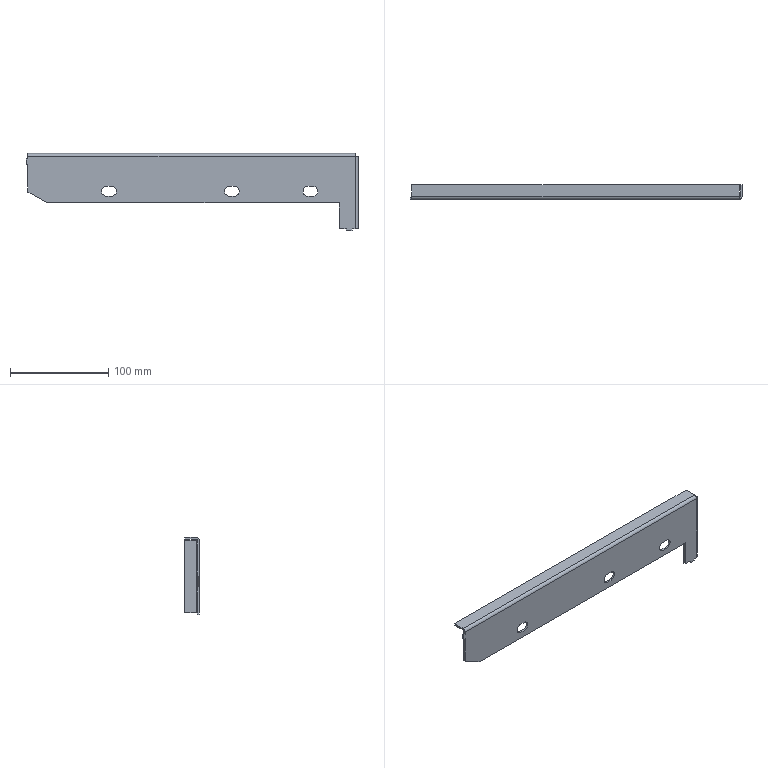Part | SolidWorks | features ICE 3, Cut 2, EdgeFlange 2, FlatPattern 1, SMBaseFlange 1, SheetMetal 1 | 1 solid | 45 faces | box 338 x 15 x 78.5 mm | volume 43707 mm3 | plane 35 | cylinder 10 | commonest cylinder face diameters 10 x6 2 x2 6 x2
STEP:
#1=CARTESIAN_POINT('',(-16.,0.,0.));
#2=VERTEX_POINT('',#1);
#3=CARTESIAN_POINT('',(-9.,0.,0.));
#4=VERTEX_POINT('',#3);
#5=CARTESIAN_POINT('',(-333.,0.,0.));
#6=DIRECTION('',(1.,0.,0.));
#7=VECTOR('',#6,1000.);
#8=LINE('',#5,#7);
#9=EDGE_CURVE('',#2,#4,#8,.T.);
#10=ORIENTED_EDGE('',*,*,#9,.T.);
#11=CARTESIAN_POINT('',(-9.,-2.,0.));
#12=VERTEX_POINT('',#11);
#13=CARTESIAN_POINT('',(-9.,0.,0.));
#14=DIRECTION('',(0.,1.,0.));
#15=VECTOR('',#14,1000.);
#16=LINE('',#13,#15);
#17=EDGE_CURVE('',#12,#4,#16,.T.);
#18=ORIENTED_EDGE('',*,*,#17,.F.);
#19=CARTESIAN_POINT('',(-16.,-2.,0.));
#20=VERTEX_POINT('',#19);
#21=CARTESIAN_POINT('',(-333.,-2.,0.));
#22=DIRECTION('',(1.,0.,0.));
#23=VECTOR('',#22,1000.);
#24=LINE('',#21,#23);
#25=EDGE_CURVE('',#20,#12,#24,.T.);
#26=ORIENTED_EDGE('',*,*,#25,.F.);
#27=CARTESIAN_POINT('',(-16.,0.,0.));
#28=DIRECTION('',(0.,-1.,0.));
#29=VECTOR('',#28,1000.);
#30=LINE('',#27,#29);
#31=EDGE_CURVE('',#2,#20,#30,.T.);
#32=ORIENTED_EDGE('',*,*,#31,.F.);
#33=EDGE_LOOP('',(#10,#18,#26,#32));
#34=FACE_OUTER_BOUND('',#33,.T.);
#35=CARTESIAN_POINT('',(0.,0.,0.));
#36=DIRECTION('',(0.,0.,-1.));
#37=DIRECTION('',(-1.,0.,0.));
#38=AXIS2_PLACEMENT_3D('',#35,#36,#37);
#39=PLANE('',#38);
#40=ADVANCED_FACE('',(#34),#39,.T.);
#41=CARTESIAN_POINT('',(-3.,-2.,0.));
#42=VERTEX_POINT('',#41);
#43=CARTESIAN_POINT('',(0.,-2.,0.));
#44=VERTEX_POINT('',#43);
#45=CARTESIAN_POINT('',(-333.,-2.,0.));
#46=DIRECTION('',(1.,0.,0.));
#47=VECTOR('',#46,1000.);
#48=LINE('',#45,#47);
#49=EDGE_CURVE('',#42,#44,#48,.T.);
#50=ORIENTED_EDGE('',*,*,#49,.F.);
#51=CARTESIAN_POINT('',(-3.,0.,0.));
#52=VERTEX_POINT('',#51);
#53=CARTESIAN_POINT('',(-3.,0.,0.));
#54=DIRECTION('',(0.,-1.,0.));
#55=VECTOR('',#54,1000.);
#56=LINE('',#53,#55);
#57=EDGE_CURVE('',#52,#42,#56,.T.);
#58=ORIENTED_EDGE('',*,*,#57,.F.);
#59=CARTESIAN_POINT('',(0.,0.,0.));
#60=VERTEX_POINT('',#59);
#61=CARTESIAN_POINT('',(-333.,0.,0.));
#62=DIRECTION('',(1.,0.,0.));
#63=VECTOR('',#62,1000.);
#64=LINE('',#61,#63);
#65=EDGE_CURVE('',#52,#60,#64,.T.);
#66=ORIENTED_EDGE('',*,*,#65,.T.);
#67=CARTESIAN_POINT('',(0.,0.,0.));
#68=DIRECTION('',(0.,-1.,0.));
#69=VECTOR('',#68,1000.);
#70=LINE('',#67,#69);
#71=EDGE_CURVE('',#60,#44,#70,.T.);
#72=ORIENTED_EDGE('',*,*,#71,.T.);
#73=EDGE_LOOP('',(#50,#58,#66,#72));
#74=FACE_OUTER_BOUND('',#73,.T.);
#75=CARTESIAN_POINT('',(0.,0.,0.));
#76=DIRECTION('',(0.,0.,-1.));
#77=DIRECTION('',(-1.,0.,0.));
#78=AXIS2_PLACEMENT_3D('',#75,#76,#77);
#79=PLANE('',#78);
#80=ADVANCED_FACE('',(#74),#79,.T.);
#81=CARTESIAN_POINT('',(-333.,0.,73.5));
#82=VERTEX_POINT('',#81);
#83=CARTESIAN_POINT('',(-333.,0.,71.));
#84=VERTEX_POINT('',#83);
#85=CARTESIAN_POINT('',(-333.,0.,73.5));
#86=DIRECTION('',(0.,0.,-1.));
#87=VECTOR('',#86,1000.);
#88=LINE('',#85,#87);
#89=EDGE_CURVE('',#82,#84,#88,.T.);
#90=ORIENTED_EDGE('',*,*,#89,.T.);
#91=CARTESIAN_POINT('',(-333.,-2.,71.));
#92=VERTEX_POINT('',#91);
#93=CARTESIAN_POINT('',(-333.,-2.,71.));
#94=DIRECTION('',(0.,1.,0.));
#95=VECTOR('',#94,1000.);
#96=LINE('',#93,#95);
#97=EDGE_CURVE('',#92,#84,#96,.T.);
#98=ORIENTED_EDGE('',*,*,#97,.F.);
#99=CARTESIAN_POINT('',(-333.,-2.,73.5));
#100=VERTEX_POINT('',#99);
#101=CARTESIAN_POINT('',(-333.,-2.,73.5));
#102=DIRECTION('',(0.,0.,-1.));
#103=VECTOR('',#102,1000.);
#104=LINE('',#101,#103);
#105=EDGE_CURVE('',#100,#92,#104,.T.);
#106=ORIENTED_EDGE('',*,*,#105,.F.);
#107=CARTESIAN_POINT('',(-333.,-2.,73.5));
#108=DIRECTION('',(0.,1.,0.));
#109=VECTOR('',#108,1000.);
#110=LINE('',#107,#109);
#111=EDGE_CURVE('',#100,#82,#110,.T.);
#112=ORIENTED_EDGE('',*,*,#111,.T.);
#113=EDGE_LOOP('',(#90,#98,#106,#112));
#114=FACE_OUTER_BOUND('',#113,.T.);
#115=CARTESIAN_POINT('',(-333.,-2.,73.5));
#116=DIRECTION('',(-1.,0.,0.));
#117=DIRECTION('',(0.,0.,1.));
#118=AXIS2_PLACEMENT_3D('',#115,#116,#117);
#119=PLANE('',#118);
#120=ADVANCED_FACE('',(#114),#119,.T.);
#121=CARTESIAN_POINT('',(-333.,-2.,65.));
#122=VERTEX_POINT('',#121);
#123=CARTESIAN_POINT('',(-333.,-2.,37.2));
#124=VERTEX_POINT('',#123);
#125=CARTESIAN_POINT('',(-333.,-2.,73.5));
#126=DIRECTION('',(0.,0.,-1.));
#127=VECTOR('',#126,1000.);
#128=LINE('',#125,#127);
#129=EDGE_CURVE('',#122,#124,#128,.T.);
#130=ORIENTED_EDGE('',*,*,#129,.F.);
#131=CARTESIAN_POINT('',(-333.,0.,65.));
#132=VERTEX_POINT('',#131);
#133=CARTESIAN_POINT('',(-333.,-2.,65.));
#134=DIRECTION('',(0.,-1.,0.));
#135=VECTOR('',#134,1000.);
#136=LINE('',#133,#135);
#137=EDGE_CURVE('',#132,#122,#136,.T.);
#138=ORIENTED_EDGE('',*,*,#137,.F.);
#139=CARTESIAN_POINT('',(-333.,0.,37.2));
#140=VERTEX_POINT('',#139);
#141=CARTESIAN_POINT('',(-333.,0.,73.5));
#142=DIRECTION('',(0.,0.,-1.));
#143=VECTOR('',#142,1000.);
#144=LINE('',#141,#143);
#145=EDGE_CURVE('',#132,#140,#144,.T.);
#146=ORIENTED_EDGE('',*,*,#145,.T.);
#147=CARTESIAN_POINT('',(-333.,8.,37.2));
#148=DIRECTION('',(0.,-1.,0.));
#149=VECTOR('',#148,1000.);
#150=LINE('',#147,#149);
#151=EDGE_CURVE('',#140,#124,#150,.T.);
#152=ORIENTED_EDGE('',*,*,#151,.T.);
#153=EDGE_LOOP('',(#130,#138,#146,#152));
#154=FACE_OUTER_BOUND('',#153,.T.);
#155=CARTESIAN_POINT('',(-333.,-2.,73.5));
#156=DIRECTION('',(-1.,0.,0.));
#157=DIRECTION('',(0.,0.,1.));
#158=AXIS2_PLACEMENT_3D('',#155,#156,#157);
#159=PLANE('',#158);
#160=ADVANCED_FACE('',(#154),#159,.T.);
#161=CARTESIAN_POINT('',(-253.,-2.,33.));
#162=VERTEX_POINT('',#161);
#163=CARTESIAN_POINT('',(-248.,-2.,33.));
#164=VERTEX_POINT('',#163);
#165=CARTESIAN_POINT('',(-253.,-2.,33.));
#166=DIRECTION('',(1.,0.,0.));
#167=VECTOR('',#166,1000.);
#168=LINE('',#165,#167);
#169=EDGE_CURVE('',#162,#164,#168,.T.);
#170=ORIENTED_EDGE('',*,*,#169,.F.);
#171=CARTESIAN_POINT('',(-253.,-2.,43.));
#172=VERTEX_POINT('',#171);
#173=CARTESIAN_POINT('',(-253.,-2.,38.));
#174=DIRECTION('',(0.,-1.,0.));
#175=DIRECTION('',(0.,0.,-1.));
#176=AXIS2_PLACEMENT_3D('',#173,#174,#175);
#177=CIRCLE('',#176,5.);
#178=EDGE_CURVE('',#172,#162,#177,.T.);
#179=ORIENTED_EDGE('',*,*,#178,.F.);
#180=CARTESIAN_POINT('',(-248.,-2.,43.));
#181=VERTEX_POINT('',#180);
#182=CARTESIAN_POINT('',(-253.,-2.,43.));
#183=DIRECTION('',(-1.,0.,0.));
#184=VECTOR('',#183,1000.);
#185=LINE('',#182,#184);
#186=EDGE_CURVE('',#181,#172,#185,.T.);
#187=ORIENTED_EDGE('',*,*,#186,.F.);
#188=CARTESIAN_POINT('',(-248.,-2.,38.));
#189=DIRECTION('',(0.,-1.,0.));
#190=DIRECTION('',(0.,0.,-1.));
#191=AXIS2_PLACEMENT_3D('',#188,#189,#190);
#192=CIRCLE('',#191,5.);
#193=EDGE_CURVE('',#164,#181,#192,.T.);
#194=ORIENTED_EDGE('',*,*,#193,.F.);
#195=EDGE_LOOP('',(#170,#179,#187,#194));
#196=FACE_BOUND('',#195,.T.);
#197=CARTESIAN_POINT('',(-128.,-2.,33.));
#198=VERTEX_POINT('',#197);
#199=CARTESIAN_POINT('',(-123.,-2.,33.));
#200=VERTEX_POINT('',#199);
#201=CARTESIAN_POINT('',(-128.,-2.,33.));
#202=DIRECTION('',(1.,0.,0.));
#203=VECTOR('',#202,1000.);
#204=LINE('',#201,#203);
#205=EDGE_CURVE('',#198,#200,#204,.T.);
#206=ORIENTED_EDGE('',*,*,#205,.F.);
#207=CARTESIAN_POINT('',(-128.,-2.,43.));
#208=VERTEX_POINT('',#207);
#209=CARTESIAN_POINT('',(-128.,-2.,38.));
#210=DIRECTION('',(0.,-1.,0.));
#211=DIRECTION('',(0.,0.,-1.));
#212=AXIS2_PLACEMENT_3D('',#209,#210,#211);
#213=CIRCLE('',#212,5.);
#214=EDGE_CURVE('',#208,#198,#213,.T.);
#215=ORIENTED_EDGE('',*,*,#214,.F.);
#216=CARTESIAN_POINT('',(-123.,-2.,43.));
#217=VERTEX_POINT('',#216);
#218=CARTESIAN_POINT('',(-128.,-2.,43.));
#219=DIRECTION('',(-1.,0.,0.));
#220=VECTOR('',#219,1000.);
#221=LINE('',#218,#220);
#222=EDGE_CURVE('',#217,#208,#221,.T.);
#223=ORIENTED_EDGE('',*,*,#222,.F.);
#224=CARTESIAN_POINT('',(-123.,-2.,38.));
#225=DIRECTION('',(0.,-1.,0.));
#226=DIRECTION('',(0.,0.,-1.));
#227=AXIS2_PLACEMENT_3D('',#224,#225,#226);
#228=CIRCLE('',#227,5.);
#229=EDGE_CURVE('',#200,#217,#228,.T.);
#230=ORIENTED_EDGE('',*,*,#229,.F.);
#231=EDGE_LOOP('',(#206,#215,#223,#230));
#232=FACE_BOUND('',#231,.T.);
#233=CARTESIAN_POINT('',(-48.,-2.,33.));
#234=VERTEX_POINT('',#233);
#235=CARTESIAN_POINT('',(-43.,-2.,33.));
#236=VERTEX_POINT('',#235);
#237=CARTESIAN_POINT('',(-48.,-2.,33.));
#238=DIRECTION('',(1.,0.,0.));
#239=VECTOR('',#238,1000.);
#240=LINE('',#237,#239);
#241=EDGE_CURVE('',#234,#236,#240,.T.);
#242=ORIENTED_EDGE('',*,*,#241,.F.);
#243=CARTESIAN_POINT('',(-48.,-2.,43.));
#244=VERTEX_POINT('',#243);
#245=CARTESIAN_POINT('',(-48.,-2.,38.));
#246=DIRECTION('',(0.,-1.,0.));
#247=DIRECTION('',(0.,0.,-1.));
#248=AXIS2_PLACEMENT_3D('',#245,#246,#247);
#249=CIRCLE('',#248,5.);
#250=EDGE_CURVE('',#244,#234,#249,.T.);
#251=ORIENTED_EDGE('',*,*,#250,.F.);
#252=CARTESIAN_POINT('',(-43.,-2.,43.));
#253=VERTEX_POINT('',#252);
#254=CARTESIAN_POINT('',(-48.,-2.,43.));
#255=DIRECTION('',(-1.,0.,0.));
#256=VECTOR('',#255,1000.);
#257=LINE('',#254,#256);
#258=EDGE_CURVE('',#253,#244,#257,.T.);
#259=ORIENTED_EDGE('',*,*,#258,.F.);
#260=CARTESIAN_POINT('',(-43.,-2.,38.));
#261=DIRECTION('',(0.,-1.,0.));
#262=DIRECTION('',(0.,0.,-1.));
#263=AXIS2_PLACEMENT_3D('',#260,#261,#262);
#264=CIRCLE('',#263,5.);
#265=EDGE_CURVE('',#236,#253,#264,.T.);
#266=ORIENTED_EDGE('',*,*,#265,.F.);
#267=EDGE_LOOP('',(#242,#251,#259,#266));
#268=FACE_BOUND('',#267,.T.);
#269=ORIENTED_EDGE('',*,*,#105,.T.);
#270=CARTESIAN_POINT('',(-335.,-2.,71.));
#271=VERTEX_POINT('',#270);
#272=CARTESIAN_POINT('',(-335.,-2.,71.));
#273=DIRECTION('',(1.,0.,0.));
#274=VECTOR('',#273,1000.);
#275=LINE('',#272,#274);
#276=EDGE_CURVE('',#271,#92,#275,.T.);
#277=ORIENTED_EDGE('',*,*,#276,.F.);
#278=CARTESIAN_POINT('',(-335.,-2.,65.));
#279=VERTEX_POINT('',#278);
#280=CARTESIAN_POINT('',(-335.,-2.,71.));
#281=DIRECTION('',(0.,0.,1.));
#282=VECTOR('',#281,1000.);
#283=LINE('',#280,#282);
#284=EDGE_CURVE('',#279,#271,#283,.T.);
#285=ORIENTED_EDGE('',*,*,#284,.F.);
#286=CARTESIAN_POINT('',(-335.,-2.,65.));
#287=DIRECTION('',(1.,0.,0.));
#288=VECTOR('',#287,1000.);
#289=LINE('',#286,#288);
#290=EDGE_CURVE('',#279,#122,#289,.T.);
#291=ORIENTED_EDGE('',*,*,#290,.T.);
#292=ORIENTED_EDGE('',*,*,#129,.T.);
#293=CARTESIAN_POINT('',(-313.,-2.,26.2));
#294=VERTEX_POINT('',#293);
#295=CARTESIAN_POINT('',(-333.,-2.,37.2));
#296=DIRECTION('',(-0.8762,0.,0.4819));
#297=VECTOR('',#296,1000.);
#298=LINE('',#295,#297);
#299=EDGE_CURVE('',#294,#124,#298,.T.);
#300=ORIENTED_EDGE('',*,*,#299,.F.);
#301=CARTESIAN_POINT('',(-16.,-2.,26.2));
#302=VERTEX_POINT('',#301);
#303=CARTESIAN_POINT('',(-333.,-2.,26.2));
#304=DIRECTION('',(-1.,0.,0.));
#305=VECTOR('',#304,1000.);
#306=LINE('',#303,#305);
#307=EDGE_CURVE('',#302,#294,#306,.T.);
#308=ORIENTED_EDGE('',*,*,#307,.F.);
#309=CARTESIAN_POINT('',(-16.,-2.,0.));
#310=DIRECTION('',(0.,0.,1.));
#311=VECTOR('',#310,1000.);
#312=LINE('',#309,#311);
#313=EDGE_CURVE('',#20,#302,#312,.T.);
#314=ORIENTED_EDGE('',*,*,#313,.F.);
#315=ORIENTED_EDGE('',*,*,#25,.T.);
#316=CARTESIAN_POINT('',(-9.,-2.,-2.));
#317=VERTEX_POINT('',#316);
#318=CARTESIAN_POINT('',(-9.,-2.,-2.));
#319=DIRECTION('',(0.,0.,1.));
#320=VECTOR('',#319,1000.);
#321=LINE('',#318,#320);
#322=EDGE_CURVE('',#317,#12,#321,.T.);
#323=ORIENTED_EDGE('',*,*,#322,.F.);
#324=CARTESIAN_POINT('',(-3.,-2.,-2.));
#325=VERTEX_POINT('',#324);
#326=CARTESIAN_POINT('',(-9.,-2.,-2.));
#327=DIRECTION('',(-1.,0.,0.));
#328=VECTOR('',#327,1000.);
#329=LINE('',#326,#328);
#330=EDGE_CURVE('',#325,#317,#329,.T.);
#331=ORIENTED_EDGE('',*,*,#330,.F.);
#332=CARTESIAN_POINT('',(-3.,-2.,-2.));
#333=DIRECTION('',(0.,0.,1.));
#334=VECTOR('',#333,1000.);
#335=LINE('',#332,#334);
#336=EDGE_CURVE('',#325,#42,#335,.T.);
#337=ORIENTED_EDGE('',*,*,#336,.T.);
#338=ORIENTED_EDGE('',*,*,#49,.T.);
#339=CARTESIAN_POINT('',(0.,-2.,73.5));
#340=VERTEX_POINT('',#339);
#341=CARTESIAN_POINT('',(0.,-2.,73.5));
#342=DIRECTION('',(0.,0.,-1.));
#343=VECTOR('',#342,1000.);
#344=LINE('',#341,#343);
#345=EDGE_CURVE('',#340,#44,#344,.T.);
#346=ORIENTED_EDGE('',*,*,#345,.F.);
#347=CARTESIAN_POINT('',(-333.,-2.,73.5));
#348=DIRECTION('',(1.,0.,0.));
#349=VECTOR('',#348,1000.);
#350=LINE('',#347,#349);
#351=EDGE_CURVE('',#100,#340,#350,.T.);
#352=ORIENTED_EDGE('',*,*,#351,.F.);
#353=EDGE_LOOP('',(#269,#277,#285,#291,#292,#300,#308,#314,#315,#323,#331,#337,#338,#346,#352));
#354=FACE_OUTER_BOUND('',#353,.T.);
#355=CARTESIAN_POINT('',(-333.,-2.,73.5));
#356=DIRECTION('',(0.,1.,0.));
#357=DIRECTION('',(0.,0.,1.));
#358=AXIS2_PLACEMENT_3D('',#355,#356,#357);
#359=PLANE('',#358);
#360=ADVANCED_FACE('',(#196,#232,#268,#354),#359,.F.);
#361=CARTESIAN_POINT('',(-313.,0.,26.2));
#362=VERTEX_POINT('',#361);
#363=CARTESIAN_POINT('',(-348.328,0.,45.631));
#364=DIRECTION('',(0.8762,0.,-0.4819));
#365=VECTOR('',#364,1000.);
#366=LINE('',#363,#365);
#367=EDGE_CURVE('',#140,#362,#366,.T.);
#368=ORIENTED_EDGE('',*,*,#367,.F.);
#369=ORIENTED_EDGE('',*,*,#145,.F.);
#370=CARTESIAN_POINT('',(-335.,0.,65.));
#371=VERTEX_POINT('',#370);
#372=CARTESIAN_POINT('',(-335.,0.,65.));
#373=DIRECTION('',(1.,0.,0.));
#374=VECTOR('',#373,1000.);
#375=LINE('',#372,#374);
#376=EDGE_CURVE('',#371,#132,#375,.T.);
#377=ORIENTED_EDGE('',*,*,#376,.F.);
#378=CARTESIAN_POINT('',(-335.,0.,71.));
#379=VERTEX_POINT('',#378);
#380=CARTESIAN_POINT('',(-335.,0.,71.));
#381=DIRECTION('',(0.,0.,-1.));
#382=VECTOR('',#381,1000.);
#383=LINE('',#380,#382);
#384=EDGE_CURVE('',#379,#371,#383,.T.);
#385=ORIENTED_EDGE('',*,*,#384,.F.);
#386=CARTESIAN_POINT('',(-335.,0.,71.));
#387=DIRECTION('',(1.,0.,0.));
#388=VECTOR('',#387,1000.);
#389=LINE('',#386,#388);
#390=EDGE_CURVE('',#379,#84,#389,.T.);
#391=ORIENTED_EDGE('',*,*,#390,.T.);
#392=ORIENTED_EDGE('',*,*,#89,.F.);
#393=CARTESIAN_POINT('',(0.,0.,73.5));
#394=VERTEX_POINT('',#393);
#395=CARTESIAN_POINT('',(-333.,0.,73.5));
#396=DIRECTION('',(1.,0.,0.));
#397=VECTOR('',#396,1000.);
#398=LINE('',#395,#397);
#399=EDGE_CURVE('',#82,#394,#398,.T.);
#400=ORIENTED_EDGE('',*,*,#399,.T.);
#401=CARTESIAN_POINT('',(0.,0.,73.5));
#402=DIRECTION('',(0.,0.,-1.));
#403=VECTOR('',#402,1000.);
#404=LINE('',#401,#403);
#405=EDGE_CURVE('',#394,#60,#404,.T.);
#406=ORIENTED_EDGE('',*,*,#405,.T.);
#407=ORIENTED_EDGE('',*,*,#65,.F.);
#408=CARTESIAN_POINT('',(-3.,0.,-2.));
#409=VERTEX_POINT('',#408);
#410=CARTESIAN_POINT('',(-3.,0.,-2.));
#411=DIRECTION('',(0.,0.,1.));
#412=VECTOR('',#411,1000.);
#413=LINE('',#410,#412);
#414=EDGE_CURVE('',#409,#52,#413,.T.);
#415=ORIENTED_EDGE('',*,*,#414,.F.);
#416=CARTESIAN_POINT('',(-9.,0.,-2.));
#417=VERTEX_POINT('',#416);
#418=CARTESIAN_POINT('',(-9.,0.,-2.));
#419=DIRECTION('',(1.,0.,0.));
#420=VECTOR('',#419,1000.);
#421=LINE('',#418,#420);
#422=EDGE_CURVE('',#417,#409,#421,.T.);
#423=ORIENTED_EDGE('',*,*,#422,.F.);
#424=CARTESIAN_POINT('',(-9.,0.,-2.));
#425=DIRECTION('',(0.,0.,1.));
#426=VECTOR('',#425,1000.);
#427=LINE('',#424,#426);
#428=EDGE_CURVE('',#417,#4,#427,.T.);
#429=ORIENTED_EDGE('',*,*,#428,.T.);
#430=ORIENTED_EDGE('',*,*,#9,.F.);
#431=CARTESIAN_POINT('',(-16.,0.,26.2));
#432=VERTEX_POINT('',#431);
#433=CARTESIAN_POINT('',(-16.,0.,73.5));
#434=DIRECTION('',(0.,0.,-1.));
#435=VECTOR('',#434,1000.);
#436=LINE('',#433,#435);
#437=EDGE_CURVE('',#432,#2,#436,.T.);
#438=ORIENTED_EDGE('',*,*,#437,.F.);
#439=CARTESIAN_POINT('',(-333.,0.,26.2));
#440=DIRECTION('',(1.,0.,0.));
#441=VECTOR('',#440,1000.);
#442=LINE('',#439,#441);
#443=EDGE_CURVE('',#362,#432,#442,.T.);
#444=ORIENTED_EDGE('',*,*,#443,.F.);
#445=EDGE_LOOP('',(#368,#369,#377,#385,#391,#392,#400,#406,#407,#415,#423,#429,#430,#438,#444));
#446=FACE_OUTER_BOUND('',#445,.T.);
#447=CARTESIAN_POINT('',(-253.,0.,33.));
#448=VERTEX_POINT('',#447);
#449=CARTESIAN_POINT('',(-253.,0.,43.));
#450=VERTEX_POINT('',#449);
#451=CARTESIAN_POINT('',(-253.,0.,38.));
#452=DIRECTION('',(0.,1.,0.));
#453=DIRECTION('',(0.,0.,1.));
#454=AXIS2_PLACEMENT_3D('',#451,#452,#453);
#455=CIRCLE('',#454,5.);
#456=EDGE_CURVE('',#448,#450,#455,.T.);
#457=ORIENTED_EDGE('',*,*,#456,.F.);
#458=CARTESIAN_POINT('',(-248.,0.,33.));
#459=VERTEX_POINT('',#458);
#460=CARTESIAN_POINT('',(-333.,0.,33.));
#461=DIRECTION('',(-1.,0.,0.));
#462=VECTOR('',#461,1000.);
#463=LINE('',#460,#462);
#464=EDGE_CURVE('',#459,#448,#463,.T.);
#465=ORIENTED_EDGE('',*,*,#464,.F.);
#466=CARTESIAN_POINT('',(-248.,0.,43.));
#467=VERTEX_POINT('',#466);
#468=CARTESIAN_POINT('',(-248.,0.,38.));
#469=DIRECTION('',(0.,1.,0.));
#470=DIRECTION('',(0.,0.,1.));
#471=AXIS2_PLACEMENT_3D('',#468,#469,#470);
#472=CIRCLE('',#471,5.);
#473=EDGE_CURVE('',#467,#459,#472,.T.);
#474=ORIENTED_EDGE('',*,*,#473,.F.);
#475=CARTESIAN_POINT('',(-333.,0.,43.));
#476=DIRECTION('',(1.,0.,0.));
#477=VECTOR('',#476,1000.);
#478=LINE('',#475,#477);
#479=EDGE_CURVE('',#450,#467,#478,.T.);
#480=ORIENTED_EDGE('',*,*,#479,.F.);
#481=EDGE_LOOP('',(#457,#465,#474,#480));
#482=FACE_BOUND('',#481,.T.);
#483=CARTESIAN_POINT('',(-128.,0.,33.));
#484=VERTEX_POINT('',#483);
#485=CARTESIAN_POINT('',(-128.,0.,43.));
#486=VERTEX_POINT('',#485);
#487=CARTESIAN_POINT('',(-128.,0.,38.));
#488=DIRECTION('',(0.,1.,0.));
#489=DIRECTION('',(0.,0.,1.));
#490=AXIS2_PLACEMENT_3D('',#487,#488,#489);
#491=CIRCLE('',#490,5.);
#492=EDGE_CURVE('',#484,#486,#491,.T.);
#493=ORIENTED_EDGE('',*,*,#492,.F.);
#494=CARTESIAN_POINT('',(-123.,0.,33.));
#495=VERTEX_POINT('',#494);
#496=CARTESIAN_POINT('',(-333.,0.,33.));
#497=DIRECTION('',(-1.,0.,0.));
#498=VECTOR('',#497,1000.);
#499=LINE('',#496,#498);
#500=EDGE_CURVE('',#495,#484,#499,.T.);
#501=ORIENTED_EDGE('',*,*,#500,.F.);
#502=CARTESIAN_POINT('',(-123.,0.,43.));
#503=VERTEX_POINT('',#502);
#504=CARTESIAN_POINT('',(-123.,0.,38.));
#505=DIRECTION('',(0.,1.,0.));
#506=DIRECTION('',(0.,0.,1.));
#507=AXIS2_PLACEMENT_3D('',#504,#505,#506);
#508=CIRCLE('',#507,5.);
#509=EDGE_CURVE('',#503,#495,#508,.T.);
#510=ORIENTED_EDGE('',*,*,#509,.F.);
#511=CARTESIAN_POINT('',(-333.,0.,43.));
#512=DIRECTION('',(1.,0.,0.));
#513=VECTOR('',#512,1000.);
#514=LINE('',#511,#513);
#515=EDGE_CURVE('',#486,#503,#514,.T.);
#516=ORIENTED_EDGE('',*,*,#515,.F.);
#517=EDGE_LOOP('',(#493,#501,#510,#516));
#518=FACE_BOUND('',#517,.T.);
#519=CARTESIAN_POINT('',(-48.,0.,33.));
#520=VERTEX_POINT('',#519);
#521=CARTESIAN_POINT('',(-48.,0.,43.));
#522=VERTEX_POINT('',#521);
#523=CARTESIAN_POINT('',(-48.,0.,38.));
#524=DIRECTION('',(0.,1.,0.));
#525=DIRECTION('',(0.,0.,1.));
#526=AXIS2_PLACEMENT_3D('',#523,#524,#525);
#527=CIRCLE('',#526,5.);
#528=EDGE_CURVE('',#520,#522,#527,.T.);
#529=ORIENTED_EDGE('',*,*,#528,.F.);
#530=CARTESIAN_POINT('',(-43.,0.,33.));
#531=VERTEX_POINT('',#530);
#532=CARTESIAN_POINT('',(-333.,0.,33.));
#533=DIRECTION('',(-1.,0.,0.));
#534=VECTOR('',#533,1000.);
#535=LINE('',#532,#534);
#536=EDGE_CURVE('',#531,#520,#535,.T.);
#537=ORIENTED_EDGE('',*,*,#536,.F.);
#538=CARTESIAN_POINT('',(-43.,0.,43.));
#539=VERTEX_POINT('',#538);
#540=CARTESIAN_POINT('',(-43.,0.,38.));
#541=DIRECTION('',(0.,1.,0.));
#542=DIRECTION('',(0.,0.,1.));
#543=AXIS2_PLACEMENT_3D('',#540,#541,#542);
#544=CIRCLE('',#543,5.);
#545=EDGE_CURVE('',#539,#531,#544,.T.);
#546=ORIENTED_EDGE('',*,*,#545,.F.);
#547=CARTESIAN_POINT('',(-333.,0.,43.));
#548=DIRECTION('',(1.,0.,0.));
#549=VECTOR('',#548,1000.);
#550=LINE('',#547,#549);
#551=EDGE_CURVE('',#522,#539,#550,.T.);
#552=ORIENTED_EDGE('',*,*,#551,.F.);
#553=EDGE_LOOP('',(#529,#537,#546,#552));
#554=FACE_BOUND('',#553,.T.);
#555=CARTESIAN_POINT('',(-333.,0.,73.5));
#556=DIRECTION('',(0.,1.,0.));
#557=DIRECTION('',(0.,0.,1.));
#558=AXIS2_PLACEMENT_3D('',#555,#556,#557);
#559=PLANE('',#558);
#560=ADVANCED_FACE('',(#446,#482,#518,#554),#559,.T.);
#561=CARTESIAN_POINT('',(-333.,1.,74.5));
#562=VERTEX_POINT('',#561);
#563=CARTESIAN_POINT('',(-333.,1.,76.5));
#564=VERTEX_POINT('',#563);
#565=CARTESIAN_POINT('',(-333.,1.,76.5));
#566=DIRECTION('',(0.,0.,1.));
#567=VECTOR('',#566,1000.);
#568=LINE('',#565,#567);
#569=EDGE_CURVE('',#562,#564,#568,.T.);
#570=ORIENTED_EDGE('',*,*,#569,.F.);
#571=CARTESIAN_POINT('',(-333.,1.,73.5));
#572=DIRECTION('',(-1.,0.,0.));
#573=DIRECTION('',(0.,0.,-1.));
#574=AXIS2_PLACEMENT_3D('',#571,#572,#573);
#575=CIRCLE('',#574,1.);
#576=EDGE_CURVE('',#82,#562,#575,.T.);
#577=ORIENTED_EDGE('',*,*,#576,.F.);
#578=ORIENTED_EDGE('',*,*,#111,.F.);
#579=CARTESIAN_POINT('',(-333.,1.,73.5));
#580=DIRECTION('',(-1.,0.,0.));
#581=DIRECTION('',(0.,0.,-1.));
#582=AXIS2_PLACEMENT_3D('',#579,#580,#581);
#583=CIRCLE('',#582,3.);
#584=EDGE_CURVE('',#100,#564,#583,.T.);
#585=ORIENTED_EDGE('',*,*,#584,.T.);
#586=EDGE_LOOP('',(#570,#577,#578,#585));
#587=FACE_OUTER_BOUND('',#586,.T.);
#588=CARTESIAN_POINT('',(-333.,1.,73.5));
#589=DIRECTION('',(-1.,0.,0.));
#590=DIRECTION('',(0.,0.,1.));
#591=AXIS2_PLACEMENT_3D('',#588,#589,#590);
#592=PLANE('',#591);
#593=ADVANCED_FACE('',(#587),#592,.T.);
#594=CARTESIAN_POINT('',(0.,1.,74.5));
#595=VERTEX_POINT('',#594);
#596=CARTESIAN_POINT('',(0.,1.,73.5));
#597=DIRECTION('',(1.,0.,0.));
#598=DIRECTION('',(0.,0.,-1.));
#599=AXIS2_PLACEMENT_3D('',#596,#597,#598);
#600=CIRCLE('',#599,1.);
#601=EDGE_CURVE('',#595,#394,#600,.T.);
#602=ORIENTED_EDGE('',*,*,#601,.F.);
#603=CARTESIAN_POINT('',(0.,1.,76.5));
#604=VERTEX_POINT('',#603);
#605=CARTESIAN_POINT('',(0.,1.,74.5));
#606=DIRECTION('',(0.,0.,1.));
#607=VECTOR('',#606,1000.);
#608=LINE('',#605,#607);
#609=EDGE_CURVE('',#595,#604,#608,.T.);
#610=ORIENTED_EDGE('',*,*,#609,.T.);
#611=CARTESIAN_POINT('',(0.,1.,73.5));
#612=DIRECTION('',(1.,0.,0.));
#613=DIRECTION('',(0.,0.,-1.));
#614=AXIS2_PLACEMENT_3D('',#611,#612,#613);
#615=CIRCLE('',#614,3.);
#616=EDGE_CURVE('',#604,#340,#615,.T.);
#617=ORIENTED_EDGE('',*,*,#616,.T.);
#618=CARTESIAN_POINT('',(0.,0.,73.5));
#619=DIRECTION('',(0.,-1.,0.));
#620=VECTOR('',#619,1000.);
#621=LINE('',#618,#620);
#622=EDGE_CURVE('',#394,#340,#621,.T.);
#623=ORIENTED_EDGE('',*,*,#622,.F.);
#624=EDGE_LOOP('',(#602,#610,#617,#623));
#625=FACE_OUTER_BOUND('',#624,.T.);
#626=CARTESIAN_POINT('',(0.,1.,73.5));
#627=DIRECTION('',(-1.,0.,0.));
#628=DIRECTION('',(0.,0.,1.));
#629=AXIS2_PLACEMENT_3D('',#626,#627,#628);
#630=PLANE('',#629);
#631=ADVANCED_FACE('',(#625),#630,.F.);
#632=ORIENTED_EDGE('',*,*,#351,.T.);
#633=ORIENTED_EDGE('',*,*,#616,.F.);
#634=CARTESIAN_POINT('',(-333.,1.,76.5));
#635=DIRECTION('',(-1.,0.,0.));
#636=VECTOR('',#635,1000.);
#637=LINE('',#634,#636);
#638=EDGE_CURVE('',#604,#564,#637,.T.);
#639=ORIENTED_EDGE('',*,*,#638,.T.);
#640=ORIENTED_EDGE('',*,*,#584,.F.);
#641=EDGE_LOOP('',(#632,#633,#639,#640));
#642=FACE_OUTER_BOUND('',#641,.T.);
#643=CARTESIAN_POINT('',(0.,1.,73.5));
#644=DIRECTION('',(1.,0.,0.));
#645=DIRECTION('',(0.,0.,1.));
#646=AXIS2_PLACEMENT_3D('',#643,#644,#645);
#647=CYLINDRICAL_SURFACE('',#646,3.);
#648=ADVANCED_FACE('',(#642),#647,.T.);
#649=ORIENTED_EDGE('',*,*,#399,.F.);
#650=ORIENTED_EDGE('',*,*,#576,.T.);
#651=CARTESIAN_POINT('',(-333.,1.,74.5));
#652=DIRECTION('',(1.,0.,0.));
#653=VECTOR('',#652,1000.);
#654=LINE('',#651,#653);
#655=EDGE_CURVE('',#562,#595,#654,.T.);
#656=ORIENTED_EDGE('',*,*,#655,.T.);
#657=ORIENTED_EDGE('',*,*,#601,.T.);
#658=EDGE_LOOP('',(#649,#650,#656,#657));
#659=FACE_OUTER_BOUND('',#658,.T.);
#660=CARTESIAN_POINT('',(0.,1.,73.5));
#661=DIRECTION('',(1.,0.,0.));
#662=DIRECTION('',(0.,0.,1.));
#663=AXIS2_PLACEMENT_3D('',#660,#661,#662);
#664=CYLINDRICAL_SURFACE('',#663,1.);
#665=ADVANCED_FACE('',(#659),#664,.F.);
#666=ORIENTED_EDGE('',*,*,#569,.T.);
#667=CARTESIAN_POINT('',(-333.,13.,76.5));
#668=VERTEX_POINT('',#667);
#669=CARTESIAN_POINT('',(-333.,0.,76.5));
#670=DIRECTION('',(0.,-1.,0.));
#671=VECTOR('',#670,1000.);
#672=LINE('',#669,#671);
#673=EDGE_CURVE('',#668,#564,#672,.T.);
#674=ORIENTED_EDGE('',*,*,#673,.F.);
#675=CARTESIAN_POINT('',(-333.,13.,74.5));
#676=VERTEX_POINT('',#675);
#677=CARTESIAN_POINT('',(-333.,13.,76.5));
#678=DIRECTION('',(0.,0.,-1.));
#679=VECTOR('',#678,1000.);
#680=LINE('',#677,#679);
#681=EDGE_CURVE('',#668,#676,#680,.T.);
#682=ORIENTED_EDGE('',*,*,#681,.T.);
#683=CARTESIAN_POINT('',(-333.,0.,74.5));
#684=DIRECTION('',(0.,-1.,0.));
#685=VECTOR('',#684,1000.);
#686=LINE('',#683,#685);
#687=EDGE_CURVE('',#676,#562,#686,.T.);
#688=ORIENTED_EDGE('',*,*,#687,.T.);
#689=EDGE_LOOP('',(#666,#674,#682,#688));
#690=FACE_OUTER_BOUND('',#689,.T.);
#691=CARTESIAN_POINT('',(-333.,0.,76.5));
#692=DIRECTION('',(1.,0.,0.));
#693=DIRECTION('',(0.,0.,-1.));
#694=AXIS2_PLACEMENT_3D('',#691,#692,#693);
#695=PLANE('',#694);
#696=ADVANCED_FACE('',(#690),#695,.F.);
#697=ORIENTED_EDGE('',*,*,#609,.F.);
#698=CARTESIAN_POINT('',(0.,13.,74.5));
#699=VERTEX_POINT('',#698);
#700=CARTESIAN_POINT('',(0.,13.,74.5));
#701=DIRECTION('',(0.,1.,0.));
#702=VECTOR('',#701,1000.);
#703=LINE('',#700,#702);
#704=EDGE_CURVE('',#595,#699,#703,.T.);
#705=ORIENTED_EDGE('',*,*,#704,.T.);
#706=CARTESIAN_POINT('',(0.,13.,76.5));
#707=VERTEX_POINT('',#706);
#708=CARTESIAN_POINT('',(0.,13.,76.5));
#709=DIRECTION('',(0.,0.,-1.));
#710=VECTOR('',#709,1000.);
#711=LINE('',#708,#710);
#712=EDGE_CURVE('',#707,#699,#711,.T.);
#713=ORIENTED_EDGE('',*,*,#712,.F.);
#714=CARTESIAN_POINT('',(0.,0.,76.5));
#715=DIRECTION('',(0.,1.,0.));
#716=VECTOR('',#715,1000.);
#717=LINE('',#714,#716);
#718=EDGE_CURVE('',#604,#707,#717,.T.);
#719=ORIENTED_EDGE('',*,*,#718,.F.);
#720=EDGE_LOOP('',(#697,#705,#713,#719));
#721=FACE_OUTER_BOUND('',#720,.T.);
#722=CARTESIAN_POINT('',(0.,13.,76.5));
#723=DIRECTION('',(-1.,0.,0.));
#724=DIRECTION('',(0.,0.,1.));
#725=AXIS2_PLACEMENT_3D('',#722,#723,#724);
#726=PLANE('',#725);
#727=ADVANCED_FACE('',(#721),#726,.F.);
#728=ORIENTED_EDGE('',*,*,#638,.F.);
#729=ORIENTED_EDGE('',*,*,#718,.T.);
#730=CARTESIAN_POINT('',(0.,13.,76.5));
#731=DIRECTION('',(-1.,0.,0.));
#732=VECTOR('',#731,1000.);
#733=LINE('',#730,#732);
#734=EDGE_CURVE('',#707,#668,#733,.T.);
#735=ORIENTED_EDGE('',*,*,#734,.T.);
#736=ORIENTED_EDGE('',*,*,#673,.T.);
#737=EDGE_LOOP('',(#728,#729,#735,#736));
#738=FACE_OUTER_BOUND('',#737,.T.);
#739=CARTESIAN_POINT('',(0.,0.,76.5));
#740=DIRECTION('',(0.,0.,-1.));
#741=DIRECTION('',(-1.,0.,0.));
#742=AXIS2_PLACEMENT_3D('',#739,#740,#741);
#743=PLANE('',#742);
#744=ADVANCED_FACE('',(#738),#743,.F.);
#745=ORIENTED_EDGE('',*,*,#704,.F.);
#746=ORIENTED_EDGE('',*,*,#655,.F.);
#747=ORIENTED_EDGE('',*,*,#687,.F.);
#748=CARTESIAN_POINT('',(-333.,13.,74.5));
#749=DIRECTION('',(-1.,0.,0.));
#750=VECTOR('',#749,1000.);
#751=LINE('',#748,#750);
#752=EDGE_CURVE('',#699,#676,#751,.T.);
#753=ORIENTED_EDGE('',*,*,#752,.F.);
#754=EDGE_LOOP('',(#745,#746,#747,#753));
#755=FACE_OUTER_BOUND('',#754,.T.);
#756=CARTESIAN_POINT('',(0.,0.,74.5));
#757=DIRECTION('',(0.,0.,-1.));
#758=DIRECTION('',(-1.,0.,0.));
#759=AXIS2_PLACEMENT_3D('',#756,#757,#758);
#760=PLANE('',#759);
#761=ADVANCED_FACE('',(#755),#760,.T.);
#762=ORIENTED_EDGE('',*,*,#752,.T.);
#763=ORIENTED_EDGE('',*,*,#681,.F.);
#764=ORIENTED_EDGE('',*,*,#734,.F.);
#765=ORIENTED_EDGE('',*,*,#712,.T.);
#766=EDGE_LOOP('',(#762,#763,#764,#765));
#767=FACE_OUTER_BOUND('',#766,.T.);
#768=CARTESIAN_POINT('',(-333.,13.,76.5));
#769=DIRECTION('',(0.,-1.,0.));
#770=DIRECTION('',(0.,0.,-1.));
#771=AXIS2_PLACEMENT_3D('',#768,#769,#770);
#772=PLANE('',#771);
#773=ADVANCED_FACE('',(#767),#772,.F.);
#774=CARTESIAN_POINT('',(1.,1.,73.5));
#775=VERTEX_POINT('',#774);
#776=CARTESIAN_POINT('',(3.,1.,73.5));
#777=VERTEX_POINT('',#776);
#778=CARTESIAN_POINT('',(3.,1.,73.5));
#779=DIRECTION('',(1.,0.,0.));
#780=VECTOR('',#779,1000.);
#781=LINE('',#778,#780);
#782=EDGE_CURVE('',#775,#777,#781,.T.);
#783=ORIENTED_EDGE('',*,*,#782,.F.);
#784=CARTESIAN_POINT('',(0.,1.,73.5));
#785=DIRECTION('',(0.,0.,1.));
#786=DIRECTION('',(-1.,0.,0.));
#787=AXIS2_PLACEMENT_3D('',#784,#785,#786);
#788=CIRCLE('',#787,1.);
#789=EDGE_CURVE('',#394,#775,#788,.T.);
#790=ORIENTED_EDGE('',*,*,#789,.F.);
#791=ORIENTED_EDGE('',*,*,#622,.T.);
#792=CARTESIAN_POINT('',(0.,1.,73.5));
#793=DIRECTION('',(0.,0.,1.));
#794=DIRECTION('',(-1.,0.,0.));
#795=AXIS2_PLACEMENT_3D('',#792,#793,#794);
#796=CIRCLE('',#795,3.);
#797=EDGE_CURVE('',#340,#777,#796,.T.);
#798=ORIENTED_EDGE('',*,*,#797,.T.);
#799=EDGE_LOOP('',(#783,#790,#791,#798));
#800=FACE_OUTER_BOUND('',#799,.T.);
#801=CARTESIAN_POINT('',(0.,1.,73.5));
#802=DIRECTION('',(0.,0.,1.));
#803=DIRECTION('',(1.,0.,0.));
#804=AXIS2_PLACEMENT_3D('',#801,#802,#803);
#805=PLANE('',#804);
#806=ADVANCED_FACE('',(#800),#805,.T.);
#807=CARTESIAN_POINT('',(1.,1.,0.));
#808=VERTEX_POINT('',#807);
#809=CARTESIAN_POINT('',(0.,1.,0.));
#810=DIRECTION('',(0.,0.,-1.));
#811=DIRECTION('',(-1.,0.,0.));
#812=AXIS2_PLACEMENT_3D('',#809,#810,#811);
#813=CIRCLE('',#812,1.);
#814=EDGE_CURVE('',#808,#60,#813,.T.);
#815=ORIENTED_EDGE('',*,*,#814,.F.);
#816=CARTESIAN_POINT('',(3.,1.,0.));
#817=VERTEX_POINT('',#816);
#818=CARTESIAN_POINT('',(1.,1.,0.));
#819=DIRECTION('',(1.,0.,0.));
#820=VECTOR('',#819,1000.);
#821=LINE('',#818,#820);
#822=EDGE_CURVE('',#808,#817,#821,.T.);
#823=ORIENTED_EDGE('',*,*,#822,.T.);
#824=CARTESIAN_POINT('',(0.,1.,0.));
#825=DIRECTION('',(0.,0.,-1.));
#826=DIRECTION('',(-1.,0.,0.));
#827=AXIS2_PLACEMENT_3D('',#824,#825,#826);
#828=CIRCLE('',#827,3.);
#829=EDGE_CURVE('',#817,#44,#828,.T.);
#830=ORIENTED_EDGE('',*,*,#829,.T.);
#831=ORIENTED_EDGE('',*,*,#71,.F.);
#832=EDGE_LOOP('',(#815,#823,#830,#831));
#833=FACE_OUTER_BOUND('',#832,.T.);
#834=CARTESIAN_POINT('',(0.,1.,0.));
#835=DIRECTION('',(0.,0.,1.));
#836=DIRECTION('',(1.,0.,0.));
#837=AXIS2_PLACEMENT_3D('',#834,#835,#836);
#838=PLANE('',#837);
#839=ADVANCED_FACE('',(#833),#838,.F.);
#840=ORIENTED_EDGE('',*,*,#345,.T.);
#841=ORIENTED_EDGE('',*,*,#829,.F.);
#842=CARTESIAN_POINT('',(3.,1.,73.5));
#843=DIRECTION('',(0.,0.,1.));
#844=VECTOR('',#843,1000.);
#845=LINE('',#842,#844);
#846=EDGE_CURVE('',#817,#777,#845,.T.);
#847=ORIENTED_EDGE('',*,*,#846,.T.);
#848=ORIENTED_EDGE('',*,*,#797,.F.);
#849=EDGE_LOOP('',(#840,#841,#847,#848));
#850=FACE_OUTER_BOUND('',#849,.T.);
#851=CARTESIAN_POINT('',(0.,1.,0.));
#852=DIRECTION('',(0.,0.,-1.));
#853=DIRECTION('',(1.,0.,0.));
#854=AXIS2_PLACEMENT_3D('',#851,#852,#853);
#855=CYLINDRICAL_SURFACE('',#854,3.);
#856=ADVANCED_FACE('',(#850),#855,.T.);
#857=ORIENTED_EDGE('',*,*,#405,.F.);
#858=ORIENTED_EDGE('',*,*,#789,.T.);
#859=CARTESIAN_POINT('',(1.,1.,73.5));
#860=DIRECTION('',(0.,0.,-1.));
#861=VECTOR('',#860,1000.);
#862=LINE('',#859,#861);
#863=EDGE_CURVE('',#775,#808,#862,.T.);
#864=ORIENTED_EDGE('',*,*,#863,.T.);
#865=ORIENTED_EDGE('',*,*,#814,.T.);
#866=EDGE_LOOP('',(#857,#858,#864,#865));
#867=FACE_OUTER_BOUND('',#866,.T.);
#868=CARTESIAN_POINT('',(0.,1.,0.));
#869=DIRECTION('',(0.,0.,-1.));
#870=DIRECTION('',(1.,0.,0.));
#871=AXIS2_PLACEMENT_3D('',#868,#869,#870);
#872=CYLINDRICAL_SURFACE('',#871,1.);
#873=ADVANCED_FACE('',(#867),#872,.F.);
#874=ORIENTED_EDGE('',*,*,#782,.T.);
#875=CARTESIAN_POINT('',(3.,13.,73.5));
#876=VERTEX_POINT('',#875);
#877=CARTESIAN_POINT('',(3.,0.,73.5));
#878=DIRECTION('',(0.,-1.,0.));
#879=VECTOR('',#878,1000.);
#880=LINE('',#877,#879);
#881=EDGE_CURVE('',#876,#777,#880,.T.);
#882=ORIENTED_EDGE('',*,*,#881,.F.);
#883=CARTESIAN_POINT('',(1.,13.,73.5));
#884=VERTEX_POINT('',#883);
#885=CARTESIAN_POINT('',(3.,13.,73.5));
#886=DIRECTION('',(-1.,0.,0.));
#887=VECTOR('',#886,1000.);
#888=LINE('',#885,#887);
#889=EDGE_CURVE('',#876,#884,#888,.T.);
#890=ORIENTED_EDGE('',*,*,#889,.T.);
#891=CARTESIAN_POINT('',(1.,0.,73.5));
#892=DIRECTION('',(0.,-1.,0.));
#893=VECTOR('',#892,1000.);
#894=LINE('',#891,#893);
#895=EDGE_CURVE('',#884,#775,#894,.T.);
#896=ORIENTED_EDGE('',*,*,#895,.T.);
#897=EDGE_LOOP('',(#874,#882,#890,#896));
#898=FACE_OUTER_BOUND('',#897,.T.);
#899=CARTESIAN_POINT('',(3.,0.,73.5));
#900=DIRECTION('',(0.,0.,-1.));
#901=DIRECTION('',(-1.,0.,0.));
#902=AXIS2_PLACEMENT_3D('',#899,#900,#901);
#903=PLANE('',#902);
#904=ADVANCED_FACE('',(#898),#903,.F.);
#905=ORIENTED_EDGE('',*,*,#822,.F.);
#906=CARTESIAN_POINT('',(1.,13.,0.));
#907=VERTEX_POINT('',#906);
#908=CARTESIAN_POINT('',(1.,13.,0.));
#909=DIRECTION('',(0.,1.,0.));
#910=VECTOR('',#909,1000.);
#911=LINE('',#908,#910);
#912=EDGE_CURVE('',#808,#907,#911,.T.);
#913=ORIENTED_EDGE('',*,*,#912,.T.);
#914=CARTESIAN_POINT('',(3.,13.,0.));
#915=VERTEX_POINT('',#914);
#916=CARTESIAN_POINT('',(3.,13.,0.));
#917=DIRECTION('',(-1.,0.,0.));
#918=VECTOR('',#917,1000.);
#919=LINE('',#916,#918);
#920=EDGE_CURVE('',#915,#907,#919,.T.);
#921=ORIENTED_EDGE('',*,*,#920,.F.);
#922=CARTESIAN_POINT('',(3.,0.,0.));
#923=DIRECTION('',(0.,1.,0.));
#924=VECTOR('',#923,1000.);
#925=LINE('',#922,#924);
#926=EDGE_CURVE('',#817,#915,#925,.T.);
#927=ORIENTED_EDGE('',*,*,#926,.F.);
#928=EDGE_LOOP('',(#905,#913,#921,#927));
#929=FACE_OUTER_BOUND('',#928,.T.);
#930=CARTESIAN_POINT('',(3.,13.,0.));
#931=DIRECTION('',(0.,0.,1.));
#932=DIRECTION('',(1.,0.,0.));
#933=AXIS2_PLACEMENT_3D('',#930,#931,#932);
#934=PLANE('',#933);
#935=ADVANCED_FACE('',(#929),#934,.F.);
#936=ORIENTED_EDGE('',*,*,#846,.F.);
#937=ORIENTED_EDGE('',*,*,#926,.T.);
#938=CARTESIAN_POINT('',(3.,13.,0.));
#939=DIRECTION('',(0.,0.,1.));
#940=VECTOR('',#939,1000.);
#941=LINE('',#938,#940);
#942=EDGE_CURVE('',#915,#876,#941,.T.);
#943=ORIENTED_EDGE('',*,*,#942,.T.);
#944=ORIENTED_EDGE('',*,*,#881,.T.);
#945=EDGE_LOOP('',(#936,#937,#943,#944));
#946=FACE_OUTER_BOUND('',#945,.T.);
#947=CARTESIAN_POINT('',(3.,0.,0.));
#948=DIRECTION('',(-1.,0.,0.));
#949=DIRECTION('',(0.,-1.,0.));
#950=AXIS2_PLACEMENT_3D('',#947,#948,#949);
#951=PLANE('',#950);
#952=ADVANCED_FACE('',(#946),#951,.F.);
#953=ORIENTED_EDGE('',*,*,#912,.F.);
#954=ORIENTED_EDGE('',*,*,#863,.F.);
#955=ORIENTED_EDGE('',*,*,#895,.F.);
#956=CARTESIAN_POINT('',(1.,13.,73.5));
#957=DIRECTION('',(0.,0.,1.));
#958=VECTOR('',#957,1000.);
#959=LINE('',#956,#958);
#960=EDGE_CURVE('',#907,#884,#959,.T.);
#961=ORIENTED_EDGE('',*,*,#960,.F.);
#962=EDGE_LOOP('',(#953,#954,#955,#961));
#963=FACE_OUTER_BOUND('',#962,.T.);
#964=CARTESIAN_POINT('',(1.,0.,0.));
#965=DIRECTION('',(-1.,0.,0.));
#966=DIRECTION('',(0.,-1.,0.));
#967=AXIS2_PLACEMENT_3D('',#964,#965,#966);
#968=PLANE('',#967);
#969=ADVANCED_FACE('',(#963),#968,.T.);
#970=ORIENTED_EDGE('',*,*,#960,.T.);
#971=ORIENTED_EDGE('',*,*,#889,.F.);
#972=ORIENTED_EDGE('',*,*,#942,.F.);
#973=ORIENTED_EDGE('',*,*,#920,.T.);
#974=EDGE_LOOP('',(#970,#971,#972,#973));
#975=FACE_OUTER_BOUND('',#974,.T.);
#976=CARTESIAN_POINT('',(3.,13.,73.5));
#977=DIRECTION('',(0.,-1.,0.));
#978=DIRECTION('',(1.,0.,0.));
#979=AXIS2_PLACEMENT_3D('',#976,#977,#978);
#980=PLANE('',#979);
#981=ADVANCED_FACE('',(#975),#980,.F.);
#982=ORIENTED_EDGE('',*,*,#307,.T.);
#983=CARTESIAN_POINT('',(-313.,8.,26.2));
#984=DIRECTION('',(0.,1.,0.));
#985=VECTOR('',#984,1000.);
#986=LINE('',#983,#985);
#987=EDGE_CURVE('',#294,#362,#986,.T.);
#988=ORIENTED_EDGE('',*,*,#987,.T.);
#989=ORIENTED_EDGE('',*,*,#443,.T.);
#990=CARTESIAN_POINT('',(-16.,8.,26.2));
#991=DIRECTION('',(0.,-1.,0.));
#992=VECTOR('',#991,1000.);
#993=LINE('',#990,#992);
#994=EDGE_CURVE('',#432,#302,#993,.T.);
#995=ORIENTED_EDGE('',*,*,#994,.T.);
#996=EDGE_LOOP('',(#982,#988,#989,#995));
#997=FACE_OUTER_BOUND('',#996,.T.);
#998=CARTESIAN_POINT('',(-333.,8.,26.2));
#999=DIRECTION('',(0.,0.,1.));
#1000=DIRECTION('',(1.,0.,0.));
#1001=AXIS2_PLACEMENT_3D('',#998,#999,#1000);
#1002=PLANE('',#1001);
#1003=ADVANCED_FACE('',(#997),#1002,.F.);
#1004=ORIENTED_EDGE('',*,*,#437,.T.);
#1005=ORIENTED_EDGE('',*,*,#31,.T.);
#1006=ORIENTED_EDGE('',*,*,#313,.T.);
#1007=ORIENTED_EDGE('',*,*,#994,.F.);
#1008=EDGE_LOOP('',(#1004,#1005,#1006,#1007));
#1009=FACE_OUTER_BOUND('',#1008,.T.);
#1010=CARTESIAN_POINT('',(-16.,8.,0.));
#1011=DIRECTION('',(1.,0.,0.));
#1012=DIRECTION('',(0.,0.,-1.));
#1013=AXIS2_PLACEMENT_3D('',#1010,#1011,#1012);
#1014=PLANE('',#1013);
#1015=ADVANCED_FACE('',(#1009),#1014,.F.);
#1016=ORIENTED_EDGE('',*,*,#528,.T.);
#1017=CARTESIAN_POINT('',(-48.,8.,43.));
#1018=DIRECTION('',(0.,-1.,0.));
#1019=VECTOR('',#1018,1000.);
#1020=LINE('',#1017,#1019);
#1021=EDGE_CURVE('',#522,#244,#1020,.T.);
#1022=ORIENTED_EDGE('',*,*,#1021,.T.);
#1023=ORIENTED_EDGE('',*,*,#250,.T.);
#1024=CARTESIAN_POINT('',(-48.,8.,33.));
#1025=DIRECTION('',(0.,-1.,0.));
#1026=VECTOR('',#1025,1000.);
#1027=LINE('',#1024,#1026);
#1028=EDGE_CURVE('',#520,#234,#1027,.T.);
#1029=ORIENTED_EDGE('',*,*,#1028,.F.);
#1030=EDGE_LOOP('',(#1016,#1022,#1023,#1029));
#1031=FACE_OUTER_BOUND('',#1030,.T.);
#1032=CARTESIAN_POINT('',(-48.,8.,38.));
#1033=DIRECTION('',(0.,-1.,0.));
#1034=DIRECTION('',(0.,0.,-1.));
#1035=AXIS2_PLACEMENT_3D('',#1032,#1033,#1034);
#1036=CYLINDRICAL_SURFACE('',#1035,5.);
#1037=ADVANCED_FACE('',(#1031),#1036,.F.);
#1038=ORIENTED_EDGE('',*,*,#551,.T.);
#1039=CARTESIAN_POINT('',(-43.,8.,43.));
#1040=DIRECTION('',(0.,-1.,0.));
#1041=VECTOR('',#1040,1000.);
#1042=LINE('',#1039,#1041);
#1043=EDGE_CURVE('',#539,#253,#1042,.T.);
#1044=ORIENTED_EDGE('',*,*,#1043,.T.);
#1045=ORIENTED_EDGE('',*,*,#258,.T.);
#1046=ORIENTED_EDGE('',*,*,#1021,.F.);
#1047=EDGE_LOOP('',(#1038,#1044,#1045,#1046));
#1048=FACE_OUTER_BOUND('',#1047,.T.);
#1049=CARTESIAN_POINT('',(-48.,8.,43.));
#1050=DIRECTION('',(0.,0.,1.));
#1051=DIRECTION('',(1.,0.,0.));
#1052=AXIS2_PLACEMENT_3D('',#1049,#1050,#1051);
#1053=PLANE('',#1052);
#1054=ADVANCED_FACE('',(#1048),#1053,.F.);
#1055=ORIENTED_EDGE('',*,*,#545,.T.);
#1056=CARTESIAN_POINT('',(-43.,8.,33.));
#1057=DIRECTION('',(0.,-1.,0.));
#1058=VECTOR('',#1057,1000.);
#1059=LINE('',#1056,#1058);
#1060=EDGE_CURVE('',#531,#236,#1059,.T.);
#1061=ORIENTED_EDGE('',*,*,#1060,.T.);
#1062=ORIENTED_EDGE('',*,*,#265,.T.);
#1063=ORIENTED_EDGE('',*,*,#1043,.F.);
#1064=EDGE_LOOP('',(#1055,#1061,#1062,#1063));
#1065=FACE_OUTER_BOUND('',#1064,.T.);
#1066=CARTESIAN_POINT('',(-43.,8.,38.));
#1067=DIRECTION('',(0.,-1.,0.));
#1068=DIRECTION('',(0.,0.,-1.));
#1069=AXIS2_PLACEMENT_3D('',#1066,#1067,#1068);
#1070=CYLINDRICAL_SURFACE('',#1069,5.);
#1071=ADVANCED_FACE('',(#1065),#1070,.F.);
#1072=ORIENTED_EDGE('',*,*,#536,.T.);
#1073=ORIENTED_EDGE('',*,*,#1028,.T.);
#1074=ORIENTED_EDGE('',*,*,#241,.T.);
#1075=ORIENTED_EDGE('',*,*,#1060,.F.);
#1076=EDGE_LOOP('',(#1072,#1073,#1074,#1075));
#1077=FACE_OUTER_BOUND('',#1076,.T.);
#1078=CARTESIAN_POINT('',(-48.,8.,33.));
#1079=DIRECTION('',(0.,0.,-1.));
#1080=DIRECTION('',(-1.,0.,0.));
#1081=AXIS2_PLACEMENT_3D('',#1078,#1079,#1080);
#1082=PLANE('',#1081);
#1083=ADVANCED_FACE('',(#1077),#1082,.F.);
#1084=ORIENTED_EDGE('',*,*,#492,.T.);
#1085=CARTESIAN_POINT('',(-128.,8.,43.));
#1086=DIRECTION('',(0.,-1.,0.));
#1087=VECTOR('',#1086,1000.);
#1088=LINE('',#1085,#1087);
#1089=EDGE_CURVE('',#486,#208,#1088,.T.);
#1090=ORIENTED_EDGE('',*,*,#1089,.T.);
#1091=ORIENTED_EDGE('',*,*,#214,.T.);
#1092=CARTESIAN_POINT('',(-128.,8.,33.));
#1093=DIRECTION('',(0.,-1.,0.));
#1094=VECTOR('',#1093,1000.);
#1095=LINE('',#1092,#1094);
#1096=EDGE_CURVE('',#484,#198,#1095,.T.);
#1097=ORIENTED_EDGE('',*,*,#1096,.F.);
#1098=EDGE_LOOP('',(#1084,#1090,#1091,#1097));
#1099=FACE_OUTER_BOUND('',#1098,.T.);
#1100=CARTESIAN_POINT('',(-128.,8.,38.));
#1101=DIRECTION('',(0.,-1.,0.));
#1102=DIRECTION('',(0.,0.,-1.));
#1103=AXIS2_PLACEMENT_3D('',#1100,#1101,#1102);
#1104=CYLINDRICAL_SURFACE('',#1103,5.);
#1105=ADVANCED_FACE('',(#1099),#1104,.F.);
#1106=ORIENTED_EDGE('',*,*,#515,.T.);
#1107=CARTESIAN_POINT('',(-123.,8.,43.));
#1108=DIRECTION('',(0.,-1.,0.));
#1109=VECTOR('',#1108,1000.);
#1110=LINE('',#1107,#1109);
#1111=EDGE_CURVE('',#503,#217,#1110,.T.);
#1112=ORIENTED_EDGE('',*,*,#1111,.T.);
#1113=ORIENTED_EDGE('',*,*,#222,.T.);
#1114=ORIENTED_EDGE('',*,*,#1089,.F.);
#1115=EDGE_LOOP('',(#1106,#1112,#1113,#1114));
#1116=FACE_OUTER_BOUND('',#1115,.T.);
#1117=CARTESIAN_POINT('',(-128.,8.,43.));
#1118=DIRECTION('',(0.,0.,1.));
#1119=DIRECTION('',(1.,0.,0.));
#1120=AXIS2_PLACEMENT_3D('',#1117,#1118,#1119);
#1121=PLANE('',#1120);
#1122=ADVANCED_FACE('',(#1116),#1121,.F.);
#1123=ORIENTED_EDGE('',*,*,#509,.T.);
#1124=CARTESIAN_POINT('',(-123.,8.,33.));
#1125=DIRECTION('',(0.,-1.,0.));
#1126=VECTOR('',#1125,1000.);
#1127=LINE('',#1124,#1126);
#1128=EDGE_CURVE('',#495,#200,#1127,.T.);
#1129=ORIENTED_EDGE('',*,*,#1128,.T.);
#1130=ORIENTED_EDGE('',*,*,#229,.T.);
#1131=ORIENTED_EDGE('',*,*,#1111,.F.);
#1132=EDGE_LOOP('',(#1123,#1129,#1130,#1131));
#1133=FACE_OUTER_BOUND('',#1132,.T.);
#1134=CARTESIAN_POINT('',(-123.,8.,38.));
#1135=DIRECTION('',(0.,-1.,0.));
#1136=DIRECTION('',(0.,0.,-1.));
#1137=AXIS2_PLACEMENT_3D('',#1134,#1135,#1136);
#1138=CYLINDRICAL_SURFACE('',#1137,5.);
#1139=ADVANCED_FACE('',(#1133),#1138,.F.);
#1140=ORIENTED_EDGE('',*,*,#500,.T.);
#1141=ORIENTED_EDGE('',*,*,#1096,.T.);
#1142=ORIENTED_EDGE('',*,*,#205,.T.);
#1143=ORIENTED_EDGE('',*,*,#1128,.F.);
#1144=EDGE_LOOP('',(#1140,#1141,#1142,#1143));
#1145=FACE_OUTER_BOUND('',#1144,.T.);
#1146=CARTESIAN_POINT('',(-128.,8.,33.));
#1147=DIRECTION('',(0.,0.,-1.));
#1148=DIRECTION('',(-1.,0.,0.));
#1149=AXIS2_PLACEMENT_3D('',#1146,#1147,#1148);
#1150=PLANE('',#1149);
#1151=ADVANCED_FACE('',(#1145),#1150,.F.);
#1152=ORIENTED_EDGE('',*,*,#456,.T.);
#1153=CARTESIAN_POINT('',(-253.,8.,43.));
#1154=DIRECTION('',(0.,-1.,0.));
#1155=VECTOR('',#1154,1000.);
#1156=LINE('',#1153,#1155);
#1157=EDGE_CURVE('',#450,#172,#1156,.T.);
#1158=ORIENTED_EDGE('',*,*,#1157,.T.);
#1159=ORIENTED_EDGE('',*,*,#178,.T.);
#1160=CARTESIAN_POINT('',(-253.,8.,33.));
#1161=DIRECTION('',(0.,-1.,0.));
#1162=VECTOR('',#1161,1000.);
#1163=LINE('',#1160,#1162);
#1164=EDGE_CURVE('',#448,#162,#1163,.T.);
#1165=ORIENTED_EDGE('',*,*,#1164,.F.);
#1166=EDGE_LOOP('',(#1152,#1158,#1159,#1165));
#1167=FACE_OUTER_BOUND('',#1166,.T.);
#1168=CARTESIAN_POINT('',(-253.,8.,38.));
#1169=DIRECTION('',(0.,-1.,0.));
#1170=DIRECTION('',(0.,0.,-1.));
#1171=AXIS2_PLACEMENT_3D('',#1168,#1169,#1170);
#1172=CYLINDRICAL_SURFACE('',#1171,5.);
#1173=ADVANCED_FACE('',(#1167),#1172,.F.);
#1174=ORIENTED_EDGE('',*,*,#479,.T.);
#1175=CARTESIAN_POINT('',(-248.,8.,43.));
#1176=DIRECTION('',(0.,-1.,0.));
#1177=VECTOR('',#1176,1000.);
#1178=LINE('',#1175,#1177);
#1179=EDGE_CURVE('',#467,#181,#1178,.T.);
#1180=ORIENTED_EDGE('',*,*,#1179,.T.);
#1181=ORIENTED_EDGE('',*,*,#186,.T.);
#1182=ORIENTED_EDGE('',*,*,#1157,.F.);
#1183=EDGE_LOOP('',(#1174,#1180,#1181,#1182));
#1184=FACE_OUTER_BOUND('',#1183,.T.);
#1185=CARTESIAN_POINT('',(-253.,8.,43.));
#1186=DIRECTION('',(0.,0.,1.));
#1187=DIRECTION('',(1.,0.,0.));
#1188=AXIS2_PLACEMENT_3D('',#1185,#1186,#1187);
#1189=PLANE('',#1188);
#1190=ADVANCED_FACE('',(#1184),#1189,.F.);
#1191=ORIENTED_EDGE('',*,*,#473,.T.);
#1192=CARTESIAN_POINT('',(-248.,8.,33.));
#1193=DIRECTION('',(0.,-1.,0.));
#1194=VECTOR('',#1193,1000.);
#1195=LINE('',#1192,#1194);
#1196=EDGE_CURVE('',#459,#164,#1195,.T.);
#1197=ORIENTED_EDGE('',*,*,#1196,.T.);
#1198=ORIENTED_EDGE('',*,*,#193,.T.);
#1199=ORIENTED_EDGE('',*,*,#1179,.F.);
#1200=EDGE_LOOP('',(#1191,#1197,#1198,#1199));
#1201=FACE_OUTER_BOUND('',#1200,.T.);
#1202=CARTESIAN_POINT('',(-248.,8.,38.));
#1203=DIRECTION('',(0.,-1.,0.));
#1204=DIRECTION('',(0.,0.,-1.));
#1205=AXIS2_PLACEMENT_3D('',#1202,#1203,#1204);
#1206=CYLINDRICAL_SURFACE('',#1205,5.);
#1207=ADVANCED_FACE('',(#1201),#1206,.F.);
#1208=ORIENTED_EDGE('',*,*,#464,.T.);
#1209=ORIENTED_EDGE('',*,*,#1164,.T.);
#1210=ORIENTED_EDGE('',*,*,#169,.T.);
#1211=ORIENTED_EDGE('',*,*,#1196,.F.);
#1212=EDGE_LOOP('',(#1208,#1209,#1210,#1211));
#1213=FACE_OUTER_BOUND('',#1212,.T.);
#1214=CARTESIAN_POINT('',(-253.,8.,33.));
#1215=DIRECTION('',(0.,0.,-1.));
#1216=DIRECTION('',(-1.,0.,0.));
#1217=AXIS2_PLACEMENT_3D('',#1214,#1215,#1216);
#1218=PLANE('',#1217);
#1219=ADVANCED_FACE('',(#1213),#1218,.F.);
#1220=ORIENTED_EDGE('',*,*,#367,.T.);
#1221=ORIENTED_EDGE('',*,*,#987,.F.);
#1222=ORIENTED_EDGE('',*,*,#299,.T.);
#1223=ORIENTED_EDGE('',*,*,#151,.F.);
#1224=EDGE_LOOP('',(#1220,#1221,#1222,#1223));
#1225=FACE_OUTER_BOUND('',#1224,.T.);
#1226=CARTESIAN_POINT('',(-333.,8.,37.2));
#1227=DIRECTION('',(0.4819,0.,0.8762));
#1228=DIRECTION('',(0.8762,0.,-0.4819));
#1229=AXIS2_PLACEMENT_3D('',#1226,#1227,#1228);
#1230=PLANE('',#1229);
#1231=ADVANCED_FACE('',(#1225),#1230,.F.);
#1232=ORIENTED_EDGE('',*,*,#97,.T.);
#1233=ORIENTED_EDGE('',*,*,#390,.F.);
#1234=CARTESIAN_POINT('',(-335.,-2.,71.));
#1235=DIRECTION('',(0.,1.,0.));
#1236=VECTOR('',#1235,1000.);
#1237=LINE('',#1234,#1236);
#1238=EDGE_CURVE('',#271,#379,#1237,.T.);
#1239=ORIENTED_EDGE('',*,*,#1238,.F.);
#1240=ORIENTED_EDGE('',*,*,#276,.T.);
#1241=EDGE_LOOP('',(#1232,#1233,#1239,#1240));
#1242=FACE_OUTER_BOUND('',#1241,.T.);
#1243=CARTESIAN_POINT('',(-335.,-2.,71.));
#1244=DIRECTION('',(0.,0.,-1.));
#1245=DIRECTION('',(-1.,0.,0.));
#1246=AXIS2_PLACEMENT_3D('',#1243,#1244,#1245);
#1247=PLANE('',#1246);
#1248=ADVANCED_FACE('',(#1242),#1247,.F.);
#1249=ORIENTED_EDGE('',*,*,#137,.T.);
#1250=ORIENTED_EDGE('',*,*,#290,.F.);
#1251=CARTESIAN_POINT('',(-335.,-2.,65.));
#1252=DIRECTION('',(0.,-1.,0.));
#1253=VECTOR('',#1252,1000.);
#1254=LINE('',#1251,#1253);
#1255=EDGE_CURVE('',#371,#279,#1254,.T.);
#1256=ORIENTED_EDGE('',*,*,#1255,.F.);
#1257=ORIENTED_EDGE('',*,*,#376,.T.);
#1258=EDGE_LOOP('',(#1249,#1250,#1256,#1257));
#1259=FACE_OUTER_BOUND('',#1258,.T.);
#1260=CARTESIAN_POINT('',(-335.,-2.,65.));
#1261=DIRECTION('',(0.,0.,1.));
#1262=DIRECTION('',(1.,0.,0.));
#1263=AXIS2_PLACEMENT_3D('',#1260,#1261,#1262);
#1264=PLANE('',#1263);
#1265=ADVANCED_FACE('',(#1259),#1264,.F.);
#1266=ORIENTED_EDGE('',*,*,#1238,.T.);
#1267=ORIENTED_EDGE('',*,*,#384,.T.);
#1268=ORIENTED_EDGE('',*,*,#1255,.T.);
#1269=ORIENTED_EDGE('',*,*,#284,.T.);
#1270=EDGE_LOOP('',(#1266,#1267,#1268,#1269));
#1271=FACE_OUTER_BOUND('',#1270,.T.);
#1272=CARTESIAN_POINT('',(-335.,0.,0.));
#1273=DIRECTION('',(-1.,0.,0.));
#1274=DIRECTION('',(0.,0.,1.));
#1275=AXIS2_PLACEMENT_3D('',#1272,#1273,#1274);
#1276=PLANE('',#1275);
#1277=ADVANCED_FACE('',(#1271),#1276,.T.);
#1278=ORIENTED_EDGE('',*,*,#17,.T.);
#1279=ORIENTED_EDGE('',*,*,#428,.F.);
#1280=CARTESIAN_POINT('',(-9.,0.,-2.));
#1281=DIRECTION('',(0.,1.,0.));
#1282=VECTOR('',#1281,1000.);
#1283=LINE('',#1280,#1282);
#1284=EDGE_CURVE('',#317,#417,#1283,.T.);
#1285=ORIENTED_EDGE('',*,*,#1284,.F.);
#1286=ORIENTED_EDGE('',*,*,#322,.T.);
#1287=EDGE_LOOP('',(#1278,#1279,#1285,#1286));
#1288=FACE_OUTER_BOUND('',#1287,.T.);
#1289=CARTESIAN_POINT('',(-9.,0.,-2.));
#1290=DIRECTION('',(1.,0.,0.));
#1291=DIRECTION('',(0.,1.,0.));
#1292=AXIS2_PLACEMENT_3D('',#1289,#1290,#1291);
#1293=PLANE('',#1292);
#1294=ADVANCED_FACE('',(#1288),#1293,.F.);
#1295=ORIENTED_EDGE('',*,*,#57,.T.);
#1296=ORIENTED_EDGE('',*,*,#336,.F.);
#1297=CARTESIAN_POINT('',(-3.,0.,-2.));
#1298=DIRECTION('',(0.,-1.,0.));
#1299=VECTOR('',#1298,1000.);
#1300=LINE('',#1297,#1299);
#1301=EDGE_CURVE('',#409,#325,#1300,.T.);
#1302=ORIENTED_EDGE('',*,*,#1301,.F.);
#1303=ORIENTED_EDGE('',*,*,#414,.T.);
#1304=EDGE_LOOP('',(#1295,#1296,#1302,#1303));
#1305=FACE_OUTER_BOUND('',#1304,.T.);
#1306=CARTESIAN_POINT('',(-3.,0.,-2.));
#1307=DIRECTION('',(-1.,0.,0.));
#1308=DIRECTION('',(0.,0.,1.));
#1309=AXIS2_PLACEMENT_3D('',#1306,#1307,#1308);
#1310=PLANE('',#1309);
#1311=ADVANCED_FACE('',(#1305),#1310,.F.);
#1312=ORIENTED_EDGE('',*,*,#1284,.T.);
#1313=ORIENTED_EDGE('',*,*,#422,.T.);
#1314=ORIENTED_EDGE('',*,*,#1301,.T.);
#1315=ORIENTED_EDGE('',*,*,#330,.T.);
#1316=EDGE_LOOP('',(#1312,#1313,#1314,#1315));
#1317=FACE_OUTER_BOUND('',#1316,.T.);
#1318=CARTESIAN_POINT('',(0.,0.,-2.));
#1319=DIRECTION('',(0.,0.,1.));
#1320=DIRECTION('',(1.,0.,0.));
#1321=AXIS2_PLACEMENT_3D('',#1318,#1319,#1320);
#1322=PLANE('',#1321);
#1323=ADVANCED_FACE('',(#1317),#1322,.F.);
#1324=CLOSED_SHELL('',(#40,#80,#120,#160,#360,#560,#593,#631,#648,#665,#696,#727,#744,#761,#773,#806,#839,#856,#873,#904,#935,#952,#969,#981,#1003,#1015,#1037,#1054,#1071,#1083,#1105,#1122,#1139,#1151,#1173,#1190,#1207,#1219,#1231,#1248,#1265,#1277,#1294,#1311,#1323));
#1325=MANIFOLD_SOLID_BREP('',#1324);
#1326=CARTESIAN_POINT('',(0.,0.,0.));
#1327=DIRECTION('',(0.,0.,1.));
#1328=DIRECTION('',(1.,0.,0.));
#1329=AXIS2_PLACEMENT_3D('',#1326,#1327,#1328);
#1330=(LENGTH_UNIT()NAMED_UNIT(*)SI_UNIT(.MILLI.,.METRE.));
#1331=UNCERTAINTY_MEASURE_WITH_UNIT(LENGTH_MEASURE(0.00001),#1330,'','');
#1332=(NAMED_UNIT(*)PLANE_ANGLE_UNIT()SI_UNIT($,.RADIAN.));
#1333=(NAMED_UNIT(*)SI_UNIT($,.STERADIAN.)SOLID_ANGLE_UNIT());
#1334=(GEOMETRIC_REPRESENTATION_CONTEXT(3)GLOBAL_UNCERTAINTY_ASSIGNED_CONTEXT((#1331))GLOBAL_UNIT_ASSIGNED_CONTEXT((#1330,#1332,#1333))REPRESENTATION_CONTEXT('',''));
#1335=ADVANCED_BREP_SHAPE_REPRESENTATION('',(#1325,#1329),#1334);